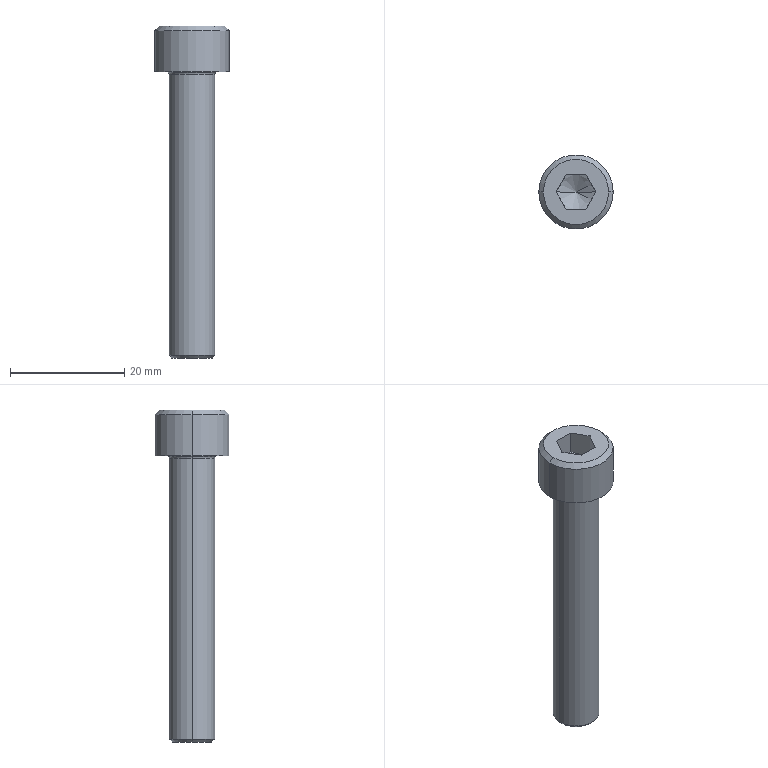Part | Creo | 1 solid | 23 faces | box 13 x 13 x 58 mm | volume 3411 mm3 | plane 9 | cone 6 | cylinder 4 | torus 4 | commonest cylinder face diameters 8 x2 13 x2
STEP:
#1=CARTESIAN_POINT('',(-230.536,192.995,-16.));
#2=VERTEX_POINT('',#1);
#3=CARTESIAN_POINT('',(-232.268,195.995,-16.));
#4=VERTEX_POINT('',#3);
#5=CARTESIAN_POINT('',(-230.536,192.995,-16.));
#6=CARTESIAN_POINT('',(-230.587,193.083,-16.029));
#7=CARTESIAN_POINT('',(-230.686,193.256,-16.083));
#8=CARTESIAN_POINT('',(-230.831,193.506,-16.149));
#9=CARTESIAN_POINT('',(-230.973,193.752,-16.201));
#10=CARTESIAN_POINT('',(-231.114,193.997,-16.239));
#11=CARTESIAN_POINT('',(-231.258,194.246,-16.263));
#12=CARTESIAN_POINT('',(-231.402,194.495,-16.271));
#13=CARTESIAN_POINT('',(-231.546,194.745,-16.263));
#14=CARTESIAN_POINT('',(-231.689,194.993,-16.239));
#15=CARTESIAN_POINT('',(-231.831,195.238,-16.201));
#16=CARTESIAN_POINT('',(-231.973,195.484,-16.149));
#17=CARTESIAN_POINT('',(-232.117,195.735,-16.083));
#18=CARTESIAN_POINT('',(-232.217,195.908,-16.029));
#19=CARTESIAN_POINT('',(-232.268,195.995,-16.));
#20=B_SPLINE_CURVE_WITH_KNOTS('',3,(#5,#6,#7,#8,#9,#10,#11,#12,#13,#14,#15,#16,#17,#18,#19),.UNSPECIFIED.,.F.,.F.,(4,1,1,1,1,1,1,1,1,1,1,1,4),(0.,0.08333,0.1667,0.25,0.3333,0.4167,0.5,0.5833,0.6667,0.75,0.8333,0.9167,1.),.UNSPECIFIED.);
#21=EDGE_CURVE('',#2,#4,#20,.T.);
#22=ORIENTED_EDGE('',*,*,#21,.F.);
#23=CARTESIAN_POINT('',(-234.,192.995,-18.));
#24=VERTEX_POINT('',#23);
#25=CARTESIAN_POINT('',(-234.,192.995,-18.));
#26=DIRECTION('',(0.866,0.,0.5));
#27=VECTOR('',#26,4.);
#28=LINE('',#25,#27);
#29=EDGE_CURVE('',#24,#2,#28,.T.);
#30=ORIENTED_EDGE('',*,*,#29,.F.);
#31=CARTESIAN_POINT('',(-237.464,192.995,-16.));
#32=VERTEX_POINT('',#31);
#33=CARTESIAN_POINT('',(-234.,192.995,-18.));
#34=DIRECTION('',(-0.866,0.,0.5));
#35=VECTOR('',#34,4.);
#36=LINE('',#33,#35);
#37=EDGE_CURVE('',#24,#32,#36,.T.);
#38=ORIENTED_EDGE('',*,*,#37,.T.);
#39=CARTESIAN_POINT('',(-235.732,195.995,-16.));
#40=VERTEX_POINT('',#39);
#41=CARTESIAN_POINT('',(-235.732,195.995,-16.));
#42=CARTESIAN_POINT('',(-235.783,195.908,-16.029));
#43=CARTESIAN_POINT('',(-235.883,195.735,-16.083));
#44=CARTESIAN_POINT('',(-236.027,195.484,-16.149));
#45=CARTESIAN_POINT('',(-236.169,195.238,-16.201));
#46=CARTESIAN_POINT('',(-236.311,194.993,-16.239));
#47=CARTESIAN_POINT('',(-236.454,194.745,-16.263));
#48=CARTESIAN_POINT('',(-236.598,194.495,-16.271));
#49=CARTESIAN_POINT('',(-236.742,194.246,-16.263));
#50=CARTESIAN_POINT('',(-236.886,193.997,-16.239));
#51=CARTESIAN_POINT('',(-237.027,193.752,-16.201));
#52=CARTESIAN_POINT('',(-237.169,193.506,-16.149));
#53=CARTESIAN_POINT('',(-237.314,193.256,-16.083));
#54=CARTESIAN_POINT('',(-237.413,193.083,-16.029));
#55=CARTESIAN_POINT('',(-237.464,192.995,-16.));
#56=B_SPLINE_CURVE_WITH_KNOTS('',3,(#41,#42,#43,#44,#45,#46,#47,#48,#49,#50,#51,#52,#53,#54,#55),.UNSPECIFIED.,.F.,.F.,(4,1,1,1,1,1,1,1,1,1,1,1,4),(0.,0.08333,0.1667,0.25,0.3333,0.4167,0.5,0.5833,0.6667,0.75,0.8333,0.9167,1.),.UNSPECIFIED.);
#57=EDGE_CURVE('',#40,#32,#56,.T.);
#58=ORIENTED_EDGE('',*,*,#57,.F.);
#59=CARTESIAN_POINT('',(-232.268,195.995,-16.));
#60=CARTESIAN_POINT('',(-232.369,195.995,-16.029));
#61=CARTESIAN_POINT('',(-232.569,195.995,-16.083));
#62=CARTESIAN_POINT('',(-232.857,195.995,-16.149));
#63=CARTESIAN_POINT('',(-233.141,195.995,-16.201));
#64=CARTESIAN_POINT('',(-233.424,195.995,-16.239));
#65=CARTESIAN_POINT('',(-233.711,195.995,-16.263));
#66=CARTESIAN_POINT('',(-234.,195.995,-16.271));
#67=CARTESIAN_POINT('',(-234.289,195.995,-16.263));
#68=CARTESIAN_POINT('',(-234.576,195.995,-16.239));
#69=CARTESIAN_POINT('',(-234.859,195.995,-16.201));
#70=CARTESIAN_POINT('',(-235.143,195.995,-16.149));
#71=CARTESIAN_POINT('',(-235.431,195.995,-16.083));
#72=CARTESIAN_POINT('',(-235.631,195.995,-16.029));
#73=CARTESIAN_POINT('',(-235.732,195.995,-16.));
#74=B_SPLINE_CURVE_WITH_KNOTS('',3,(#59,#60,#61,#62,#63,#64,#65,#66,#67,#68,#69,#70,#71,#72,#73),.UNSPECIFIED.,.F.,.F.,(4,1,1,1,1,1,1,1,1,1,1,1,4),(0.,0.08333,0.1667,0.25,0.3333,0.4167,0.5,0.5833,0.6667,0.75,0.8333,0.9167,1.),.UNSPECIFIED.);
#75=EDGE_CURVE('',#4,#40,#74,.T.);
#76=ORIENTED_EDGE('',*,*,#75,.F.);
#77=EDGE_LOOP('',(#22,#30,#38,#58,#76));
#78=FACE_OUTER_BOUND('',#77,.F.);
#79=CARTESIAN_POINT('',(-234.,192.995,-16.98));
#80=DIRECTION('',(0.,0.,1.));
#81=DIRECTION('',(1.,0.,0.));
#82=AXIS2_PLACEMENT_3D('',#79,#80,#81);
#83=CONICAL_SURFACE('',#82,1.767,60.);
#84=ADVANCED_FACE('',(#78),#83,.F.);
#85=CARTESIAN_POINT('',(-232.268,195.995,-12.));
#86=VERTEX_POINT('',#85);
#87=CARTESIAN_POINT('',(-230.536,192.995,-12.));
#88=VERTEX_POINT('',#87);
#89=CARTESIAN_POINT('',(-232.268,195.995,-12.));
#90=DIRECTION('',(0.5,-0.866,0.));
#91=VECTOR('',#90,3.464);
#92=LINE('',#89,#91);
#93=EDGE_CURVE('',#86,#88,#92,.T.);
#94=ORIENTED_EDGE('',*,*,#93,.T.);
#95=CARTESIAN_POINT('',(-230.536,192.995,-12.));
#96=DIRECTION('',(0.,0.,-1.));
#97=VECTOR('',#96,4.);
#98=LINE('',#95,#97);
#99=EDGE_CURVE('',#88,#2,#98,.T.);
#100=ORIENTED_EDGE('',*,*,#99,.T.);
#101=ORIENTED_EDGE('',*,*,#21,.T.);
#102=CARTESIAN_POINT('',(-232.268,195.995,-12.));
#103=DIRECTION('',(0.,0.,-1.));
#104=VECTOR('',#103,4.);
#105=LINE('',#102,#104);
#106=EDGE_CURVE('',#86,#4,#105,.T.);
#107=ORIENTED_EDGE('',*,*,#106,.F.);
#108=EDGE_LOOP('',(#94,#100,#101,#107));
#109=FACE_OUTER_BOUND('',#108,.F.);
#110=CARTESIAN_POINT('',(-232.268,195.995,-16.));
#111=DIRECTION('',(-0.866,-0.5,0.));
#112=DIRECTION('',(0.5,-0.866,0.));
#113=AXIS2_PLACEMENT_3D('',#110,#111,#112);
#114=PLANE('',#113);
#115=ADVANCED_FACE('',(#109),#114,.T.);
#116=CARTESIAN_POINT('',(-228.3,192.995,-12.));
#117=VERTEX_POINT('',#116);
#118=CARTESIAN_POINT('',(-239.7,192.995,-12.));
#119=VERTEX_POINT('',#118);
#120=CARTESIAN_POINT('',(-234.,192.995,-12.));
#121=DIRECTION('',(0.,0.,1.));
#122=DIRECTION('',(1.,0.,0.));
#123=AXIS2_PLACEMENT_3D('',#120,#121,#122);
#124=CIRCLE('',#123,5.7);
#125=EDGE_CURVE('',#117,#119,#124,.T.);
#126=ORIENTED_EDGE('',*,*,#125,.F.);
#127=CARTESIAN_POINT('',(-234.,192.995,-12.));
#128=DIRECTION('',(0.,0.,1.));
#129=DIRECTION('',(-1.,0.,0.));
#130=AXIS2_PLACEMENT_3D('',#127,#128,#129);
#131=CIRCLE('',#130,5.7);
#132=EDGE_CURVE('',#119,#117,#131,.T.);
#133=ORIENTED_EDGE('',*,*,#132,.F.);
#134=EDGE_LOOP('',(#126,#133));
#135=FACE_OUTER_BOUND('',#134,.F.);
#136=CARTESIAN_POINT('',(-232.268,189.995,-12.));
#137=VERTEX_POINT('',#136);
#138=CARTESIAN_POINT('',(-230.536,192.995,-12.));
#139=DIRECTION('',(-0.5,-0.866,0.));
#140=VECTOR('',#139,3.464);
#141=LINE('',#138,#140);
#142=EDGE_CURVE('',#88,#137,#141,.T.);
#143=ORIENTED_EDGE('',*,*,#142,.F.);
#144=ORIENTED_EDGE('',*,*,#93,.F.);
#145=CARTESIAN_POINT('',(-235.732,195.995,-12.));
#146=VERTEX_POINT('',#145);
#147=CARTESIAN_POINT('',(-232.268,195.995,-12.));
#148=DIRECTION('',(-1.,0.,0.));
#149=VECTOR('',#148,3.464);
#150=LINE('',#147,#149);
#151=EDGE_CURVE('',#86,#146,#150,.T.);
#152=ORIENTED_EDGE('',*,*,#151,.T.);
#153=CARTESIAN_POINT('',(-237.464,192.995,-12.));
#154=VERTEX_POINT('',#153);
#155=CARTESIAN_POINT('',(-237.464,192.995,-12.));
#156=DIRECTION('',(0.5,0.866,0.));
#157=VECTOR('',#156,3.464);
#158=LINE('',#155,#157);
#159=EDGE_CURVE('',#154,#146,#158,.T.);
#160=ORIENTED_EDGE('',*,*,#159,.F.);
#161=CARTESIAN_POINT('',(-235.732,189.995,-12.));
#162=VERTEX_POINT('',#161);
#163=CARTESIAN_POINT('',(-235.732,189.995,-12.));
#164=DIRECTION('',(-0.5,0.866,0.));
#165=VECTOR('',#164,3.464);
#166=LINE('',#163,#165);
#167=EDGE_CURVE('',#162,#154,#166,.T.);
#168=ORIENTED_EDGE('',*,*,#167,.F.);
#169=CARTESIAN_POINT('',(-235.732,189.995,-12.));
#170=DIRECTION('',(1.,0.,0.));
#171=VECTOR('',#170,3.464);
#172=LINE('',#169,#171);
#173=EDGE_CURVE('',#162,#137,#172,.T.);
#174=ORIENTED_EDGE('',*,*,#173,.T.);
#175=EDGE_LOOP('',(#143,#144,#152,#160,#168,#174));
#176=FACE_BOUND('',#175,.F.);
#177=CARTESIAN_POINT('',(-234.,192.995,-12.));
#178=DIRECTION('',(0.,0.,1.));
#179=DIRECTION('',(1.,0.,0.));
#180=AXIS2_PLACEMENT_3D('',#177,#178,#179);
#181=PLANE('',#180);
#182=ADVANCED_FACE('',(#135,#176),#181,.T.);
#183=CARTESIAN_POINT('',(-227.5,192.995,-12.8));
#184=VERTEX_POINT('',#183);
#185=CARTESIAN_POINT('',(-240.5,192.995,-12.8));
#186=VERTEX_POINT('',#185);
#187=CARTESIAN_POINT('',(-234.,192.995,-12.8));
#188=DIRECTION('',(0.,0.,1.));
#189=DIRECTION('',(1.,0.,0.));
#190=AXIS2_PLACEMENT_3D('',#187,#188,#189);
#191=CIRCLE('',#190,6.5);
#192=EDGE_CURVE('',#184,#186,#191,.T.);
#193=ORIENTED_EDGE('',*,*,#192,.F.);
#194=CARTESIAN_POINT('',(-228.3,192.995,-12.));
#195=DIRECTION('',(0.7071,0.,-0.7071));
#196=VECTOR('',#195,1.131);
#197=LINE('',#194,#196);
#198=EDGE_CURVE('',#117,#184,#197,.T.);
#199=ORIENTED_EDGE('',*,*,#198,.F.);
#200=ORIENTED_EDGE('',*,*,#125,.T.);
#201=CARTESIAN_POINT('',(-239.7,192.995,-12.));
#202=DIRECTION('',(-0.7071,0.,-0.7071));
#203=VECTOR('',#202,1.131);
#204=LINE('',#201,#203);
#205=EDGE_CURVE('',#119,#186,#204,.T.);
#206=ORIENTED_EDGE('',*,*,#205,.T.);
#207=EDGE_LOOP('',(#193,#199,#200,#206));
#208=FACE_OUTER_BOUND('',#207,.F.);
#209=CARTESIAN_POINT('',(-234.,192.995,-12.4));
#210=DIRECTION('',(0.,0.,-1.));
#211=DIRECTION('',(-1.,0.,0.));
#212=AXIS2_PLACEMENT_3D('',#209,#210,#211);
#213=CONICAL_SURFACE('',#212,6.1,45.);
#214=ADVANCED_FACE('',(#208),#213,.T.);
#215=ORIENTED_EDGE('',*,*,#192,.T.);
#216=CARTESIAN_POINT('',(-240.5,192.995,-20.));
#217=VERTEX_POINT('',#216);
#218=CARTESIAN_POINT('',(-240.5,192.995,-20.));
#219=DIRECTION('',(0.,0.,1.));
#220=VECTOR('',#219,7.2);
#221=LINE('',#218,#220);
#222=EDGE_CURVE('',#217,#186,#221,.T.);
#223=ORIENTED_EDGE('',*,*,#222,.F.);
#224=CARTESIAN_POINT('',(-227.5,192.995,-20.));
#225=VERTEX_POINT('',#224);
#226=CARTESIAN_POINT('',(-234.,192.995,-20.));
#227=DIRECTION('',(0.,0.,-1.));
#228=DIRECTION('',(-1.,0.,0.));
#229=AXIS2_PLACEMENT_3D('',#226,#227,#228);
#230=CIRCLE('',#229,6.5);
#231=EDGE_CURVE('',#217,#225,#230,.T.);
#232=ORIENTED_EDGE('',*,*,#231,.T.);
#233=CARTESIAN_POINT('',(-227.5,192.995,-20.));
#234=DIRECTION('',(0.,0.,1.));
#235=VECTOR('',#234,7.2);
#236=LINE('',#233,#235);
#237=EDGE_CURVE('',#225,#184,#236,.T.);
#238=ORIENTED_EDGE('',*,*,#237,.T.);
#239=EDGE_LOOP('',(#215,#223,#232,#238));
#240=FACE_OUTER_BOUND('',#239,.F.);
#241=CARTESIAN_POINT('',(-234.,192.995,-20.));
#242=DIRECTION('',(0.,0.,1.));
#243=DIRECTION('',(1.,0.,0.));
#244=AXIS2_PLACEMENT_3D('',#241,#242,#243);
#245=CYLINDRICAL_SURFACE('',#244,6.5);
#246=ADVANCED_FACE('',(#240),#245,.T.);
#247=CARTESIAN_POINT('',(-234.,192.995,-12.8));
#248=DIRECTION('',(0.,0.,1.));
#249=DIRECTION('',(-1.,0.,0.));
#250=AXIS2_PLACEMENT_3D('',#247,#248,#249);
#251=CIRCLE('',#250,6.5);
#252=EDGE_CURVE('',#186,#184,#251,.T.);
#253=ORIENTED_EDGE('',*,*,#252,.T.);
#254=ORIENTED_EDGE('',*,*,#237,.F.);
#255=CARTESIAN_POINT('',(-234.,192.995,-20.));
#256=DIRECTION('',(0.,0.,-1.));
#257=DIRECTION('',(1.,0.,0.));
#258=AXIS2_PLACEMENT_3D('',#255,#256,#257);
#259=CIRCLE('',#258,6.5);
#260=EDGE_CURVE('',#225,#217,#259,.T.);
#261=ORIENTED_EDGE('',*,*,#260,.T.);
#262=ORIENTED_EDGE('',*,*,#222,.T.);
#263=EDGE_LOOP('',(#253,#254,#261,#262));
#264=FACE_OUTER_BOUND('',#263,.F.);
#265=CARTESIAN_POINT('',(-234.,192.995,-20.));
#266=DIRECTION('',(0.,0.,1.));
#267=DIRECTION('',(1.,0.,0.));
#268=AXIS2_PLACEMENT_3D('',#265,#266,#267);
#269=CYLINDRICAL_SURFACE('',#268,6.5);
#270=ADVANCED_FACE('',(#264),#269,.T.);
#271=ORIENTED_EDGE('',*,*,#252,.F.);
#272=ORIENTED_EDGE('',*,*,#205,.F.);
#273=ORIENTED_EDGE('',*,*,#132,.T.);
#274=ORIENTED_EDGE('',*,*,#198,.T.);
#275=EDGE_LOOP('',(#271,#272,#273,#274));
#276=FACE_OUTER_BOUND('',#275,.F.);
#277=CARTESIAN_POINT('',(-234.,192.995,-12.4));
#278=DIRECTION('',(0.,0.,-1.));
#279=DIRECTION('',(-1.,0.,0.));
#280=AXIS2_PLACEMENT_3D('',#277,#278,#279);
#281=CONICAL_SURFACE('',#280,6.1,45.);
#282=ADVANCED_FACE('',(#276),#281,.T.);
#283=ORIENTED_EDGE('',*,*,#260,.F.);
#284=ORIENTED_EDGE('',*,*,#231,.F.);
#285=EDGE_LOOP('',(#283,#284));
#286=FACE_OUTER_BOUND('',#285,.F.);
#287=CARTESIAN_POINT('',(-229.6,192.995,-20.));
#288=VERTEX_POINT('',#287);
#289=CARTESIAN_POINT('',(-238.4,192.995,-20.));
#290=VERTEX_POINT('',#289);
#291=CARTESIAN_POINT('',(-234.,192.995,-20.));
#292=DIRECTION('',(0.,0.,1.));
#293=DIRECTION('',(1.,0.,0.));
#294=AXIS2_PLACEMENT_3D('',#291,#292,#293);
#295=CIRCLE('',#294,4.4);
#296=EDGE_CURVE('',#288,#290,#295,.T.);
#297=ORIENTED_EDGE('',*,*,#296,.F.);
#298=CARTESIAN_POINT('',(-234.,192.995,-20.));
#299=DIRECTION('',(0.,0.,1.));
#300=DIRECTION('',(-1.,0.,0.));
#301=AXIS2_PLACEMENT_3D('',#298,#299,#300);
#302=CIRCLE('',#301,4.4);
#303=EDGE_CURVE('',#290,#288,#302,.T.);
#304=ORIENTED_EDGE('',*,*,#303,.F.);
#305=EDGE_LOOP('',(#297,#304));
#306=FACE_BOUND('',#305,.F.);
#307=CARTESIAN_POINT('',(-234.,192.995,-20.));
#308=DIRECTION('',(0.,0.,1.));
#309=DIRECTION('',(1.,0.,0.));
#310=AXIS2_PLACEMENT_3D('',#307,#308,#309);
#311=PLANE('',#310);
#312=ADVANCED_FACE('',(#286,#306),#311,.F.);
#313=ORIENTED_EDGE('',*,*,#296,.T.);
#314=CARTESIAN_POINT('',(-238.117,192.995,-20.117));
#315=VERTEX_POINT('',#314);
#316=CARTESIAN_POINT('',(-238.4,192.995,-20.4));
#317=DIRECTION('',(0.,1.,0.));
#318=DIRECTION('',(0.,0.,1.));
#319=AXIS2_PLACEMENT_3D('',#316,#317,#318);
#320=CIRCLE('',#319,0.4);
#321=EDGE_CURVE('',#290,#315,#320,.T.);
#322=ORIENTED_EDGE('',*,*,#321,.T.);
#323=CARTESIAN_POINT('',(-229.883,192.995,-20.117));
#324=VERTEX_POINT('',#323);
#325=CARTESIAN_POINT('',(-234.,192.995,-20.117));
#326=DIRECTION('',(0.,0.,1.));
#327=DIRECTION('',(1.,0.,0.));
#328=AXIS2_PLACEMENT_3D('',#325,#326,#327);
#329=CIRCLE('',#328,4.117);
#330=EDGE_CURVE('',#324,#315,#329,.T.);
#331=ORIENTED_EDGE('',*,*,#330,.F.);
#332=CARTESIAN_POINT('',(-229.6,192.995,-20.4));
#333=DIRECTION('',(0.,-1.,0.));
#334=DIRECTION('',(0.,0.,1.));
#335=AXIS2_PLACEMENT_3D('',#332,#333,#334);
#336=CIRCLE('',#335,0.4);
#337=EDGE_CURVE('',#288,#324,#336,.T.);
#338=ORIENTED_EDGE('',*,*,#337,.F.);
#339=EDGE_LOOP('',(#313,#322,#331,#338));
#340=FACE_OUTER_BOUND('',#339,.F.);
#341=CARTESIAN_POINT('',(-234.,192.995,-20.4));
#342=DIRECTION('',(0.,0.,1.));
#343=DIRECTION('',(1.,0.,0.));
#344=AXIS2_PLACEMENT_3D('',#341,#342,#343);
#345=TOROIDAL_SURFACE('',#344,4.4,0.4);
#346=ADVANCED_FACE('',(#340),#345,.F.);
#347=ORIENTED_EDGE('',*,*,#303,.T.);
#348=ORIENTED_EDGE('',*,*,#337,.T.);
#349=CARTESIAN_POINT('',(-234.,192.995,-20.117));
#350=DIRECTION('',(0.,0.,1.));
#351=DIRECTION('',(-1.,0.,0.));
#352=AXIS2_PLACEMENT_3D('',#349,#350,#351);
#353=CIRCLE('',#352,4.117);
#354=EDGE_CURVE('',#315,#324,#353,.T.);
#355=ORIENTED_EDGE('',*,*,#354,.F.);
#356=ORIENTED_EDGE('',*,*,#321,.F.);
#357=EDGE_LOOP('',(#347,#348,#355,#356));
#358=FACE_OUTER_BOUND('',#357,.F.);
#359=CARTESIAN_POINT('',(-234.,192.995,-20.4));
#360=DIRECTION('',(0.,0.,1.));
#361=DIRECTION('',(1.,0.,0.));
#362=AXIS2_PLACEMENT_3D('',#359,#360,#361);
#363=TOROIDAL_SURFACE('',#362,4.4,0.4);
#364=ADVANCED_FACE('',(#358),#363,.F.);
#365=CARTESIAN_POINT('',(-238.,192.995,-20.4));
#366=VERTEX_POINT('',#365);
#367=CARTESIAN_POINT('',(-230.,192.995,-20.4));
#368=VERTEX_POINT('',#367);
#369=CARTESIAN_POINT('',(-234.,192.995,-20.4));
#370=DIRECTION('',(0.,0.,1.));
#371=DIRECTION('',(-1.,0.,0.));
#372=AXIS2_PLACEMENT_3D('',#369,#370,#371);
#373=CIRCLE('',#372,4.);
#374=EDGE_CURVE('',#366,#368,#373,.T.);
#375=ORIENTED_EDGE('',*,*,#374,.F.);
#376=CARTESIAN_POINT('',(-238.4,192.995,-20.4));
#377=DIRECTION('',(0.,1.,0.));
#378=DIRECTION('',(0.7071,0.,0.7071));
#379=AXIS2_PLACEMENT_3D('',#376,#377,#378);
#380=CIRCLE('',#379,0.4);
#381=EDGE_CURVE('',#315,#366,#380,.T.);
#382=ORIENTED_EDGE('',*,*,#381,.F.);
#383=ORIENTED_EDGE('',*,*,#354,.T.);
#384=CARTESIAN_POINT('',(-229.6,192.995,-20.4));
#385=DIRECTION('',(0.,-1.,0.));
#386=DIRECTION('',(-0.7071,0.,0.7071));
#387=AXIS2_PLACEMENT_3D('',#384,#385,#386);
#388=CIRCLE('',#387,0.4);
#389=EDGE_CURVE('',#324,#368,#388,.T.);
#390=ORIENTED_EDGE('',*,*,#389,.T.);
#391=EDGE_LOOP('',(#375,#382,#383,#390));
#392=FACE_OUTER_BOUND('',#391,.F.);
#393=CARTESIAN_POINT('',(-234.,192.995,-20.4));
#394=DIRECTION('',(0.,0.,1.));
#395=DIRECTION('',(1.,0.,0.));
#396=AXIS2_PLACEMENT_3D('',#393,#394,#395);
#397=TOROIDAL_SURFACE('',#396,4.4,0.4);
#398=ADVANCED_FACE('',(#392),#397,.F.);
#399=CARTESIAN_POINT('',(-230.,192.995,-69.5));
#400=VERTEX_POINT('',#399);
#401=CARTESIAN_POINT('',(-238.,192.995,-69.5));
#402=VERTEX_POINT('',#401);
#403=CARTESIAN_POINT('',(-234.,192.995,-69.5));
#404=DIRECTION('',(0.,0.,-1.));
#405=DIRECTION('',(1.,0.,0.));
#406=AXIS2_PLACEMENT_3D('',#403,#404,#405);
#407=CIRCLE('',#406,4.);
#408=EDGE_CURVE('',#400,#402,#407,.T.);
#409=ORIENTED_EDGE('',*,*,#408,.T.);
#410=CARTESIAN_POINT('',(-238.,192.995,-69.5));
#411=DIRECTION('',(0.,0.,1.));
#412=VECTOR('',#411,49.1);
#413=LINE('',#410,#412);
#414=EDGE_CURVE('',#402,#366,#413,.T.);
#415=ORIENTED_EDGE('',*,*,#414,.T.);
#416=ORIENTED_EDGE('',*,*,#374,.T.);
#417=CARTESIAN_POINT('',(-230.,192.995,-69.5));
#418=DIRECTION('',(0.,0.,1.));
#419=VECTOR('',#418,49.1);
#420=LINE('',#417,#419);
#421=EDGE_CURVE('',#400,#368,#420,.T.);
#422=ORIENTED_EDGE('',*,*,#421,.F.);
#423=EDGE_LOOP('',(#409,#415,#416,#422));
#424=FACE_OUTER_BOUND('',#423,.F.);
#425=CARTESIAN_POINT('',(-234.,192.995,-70.));
#426=DIRECTION('',(0.,0.,1.));
#427=DIRECTION('',(1.,0.,0.));
#428=AXIS2_PLACEMENT_3D('',#425,#426,#427);
#429=CYLINDRICAL_SURFACE('',#428,4.);
#430=ADVANCED_FACE('',(#424),#429,.T.);
#431=CARTESIAN_POINT('',(-230.5,192.995,-70.));
#432=VERTEX_POINT('',#431);
#433=CARTESIAN_POINT('',(-237.5,192.995,-70.));
#434=VERTEX_POINT('',#433);
#435=CARTESIAN_POINT('',(-234.,192.995,-70.));
#436=DIRECTION('',(0.,0.,-1.));
#437=DIRECTION('',(1.,0.,0.));
#438=AXIS2_PLACEMENT_3D('',#435,#436,#437);
#439=CIRCLE('',#438,3.5);
#440=EDGE_CURVE('',#432,#434,#439,.T.);
#441=ORIENTED_EDGE('',*,*,#440,.T.);
#442=CARTESIAN_POINT('',(-237.5,192.995,-70.));
#443=DIRECTION('',(-0.7071,0.,0.7071));
#444=VECTOR('',#443,0.7071);
#445=LINE('',#442,#444);
#446=EDGE_CURVE('',#434,#402,#445,.T.);
#447=ORIENTED_EDGE('',*,*,#446,.T.);
#448=ORIENTED_EDGE('',*,*,#408,.F.);
#449=CARTESIAN_POINT('',(-230.5,192.995,-70.));
#450=DIRECTION('',(0.7071,0.,0.7071));
#451=VECTOR('',#450,0.7071);
#452=LINE('',#449,#451);
#453=EDGE_CURVE('',#432,#400,#452,.T.);
#454=ORIENTED_EDGE('',*,*,#453,.F.);
#455=EDGE_LOOP('',(#441,#447,#448,#454));
#456=FACE_OUTER_BOUND('',#455,.F.);
#457=CARTESIAN_POINT('',(-234.,192.995,-69.75));
#458=DIRECTION('',(0.,0.,1.));
#459=DIRECTION('',(1.,0.,0.));
#460=AXIS2_PLACEMENT_3D('',#457,#458,#459);
#461=CONICAL_SURFACE('',#460,3.75,45.);
#462=ADVANCED_FACE('',(#456),#461,.T.);
#463=ORIENTED_EDGE('',*,*,#440,.F.);
#464=CARTESIAN_POINT('',(-234.,192.995,-70.));
#465=DIRECTION('',(0.,0.,-1.));
#466=DIRECTION('',(-1.,0.,0.));
#467=AXIS2_PLACEMENT_3D('',#464,#465,#466);
#468=CIRCLE('',#467,3.5);
#469=EDGE_CURVE('',#434,#432,#468,.T.);
#470=ORIENTED_EDGE('',*,*,#469,.F.);
#471=EDGE_LOOP('',(#463,#470));
#472=FACE_OUTER_BOUND('',#471,.F.);
#473=CARTESIAN_POINT('',(-234.,192.995,-70.));
#474=DIRECTION('',(0.,0.,1.));
#475=DIRECTION('',(1.,0.,0.));
#476=AXIS2_PLACEMENT_3D('',#473,#474,#475);
#477=PLANE('',#476);
#478=ADVANCED_FACE('',(#472),#477,.F.);
#479=ORIENTED_EDGE('',*,*,#469,.T.);
#480=ORIENTED_EDGE('',*,*,#453,.T.);
#481=CARTESIAN_POINT('',(-234.,192.995,-69.5));
#482=DIRECTION('',(0.,0.,-1.));
#483=DIRECTION('',(-1.,0.,0.));
#484=AXIS2_PLACEMENT_3D('',#481,#482,#483);
#485=CIRCLE('',#484,4.);
#486=EDGE_CURVE('',#402,#400,#485,.T.);
#487=ORIENTED_EDGE('',*,*,#486,.F.);
#488=ORIENTED_EDGE('',*,*,#446,.F.);
#489=EDGE_LOOP('',(#479,#480,#487,#488));
#490=FACE_OUTER_BOUND('',#489,.F.);
#491=CARTESIAN_POINT('',(-234.,192.995,-69.75));
#492=DIRECTION('',(0.,0.,1.));
#493=DIRECTION('',(1.,0.,0.));
#494=AXIS2_PLACEMENT_3D('',#491,#492,#493);
#495=CONICAL_SURFACE('',#494,3.75,45.);
#496=ADVANCED_FACE('',(#490),#495,.T.);
#497=ORIENTED_EDGE('',*,*,#486,.T.);
#498=ORIENTED_EDGE('',*,*,#421,.T.);
#499=CARTESIAN_POINT('',(-234.,192.995,-20.4));
#500=DIRECTION('',(0.,0.,1.));
#501=DIRECTION('',(1.,0.,0.));
#502=AXIS2_PLACEMENT_3D('',#499,#500,#501);
#503=CIRCLE('',#502,4.);
#504=EDGE_CURVE('',#368,#366,#503,.T.);
#505=ORIENTED_EDGE('',*,*,#504,.T.);
#506=ORIENTED_EDGE('',*,*,#414,.F.);
#507=EDGE_LOOP('',(#497,#498,#505,#506));
#508=FACE_OUTER_BOUND('',#507,.F.);
#509=CARTESIAN_POINT('',(-234.,192.995,-70.));
#510=DIRECTION('',(0.,0.,1.));
#511=DIRECTION('',(1.,0.,0.));
#512=AXIS2_PLACEMENT_3D('',#509,#510,#511);
#513=CYLINDRICAL_SURFACE('',#512,4.);
#514=ADVANCED_FACE('',(#508),#513,.T.);
#515=ORIENTED_EDGE('',*,*,#504,.F.);
#516=ORIENTED_EDGE('',*,*,#389,.F.);
#517=ORIENTED_EDGE('',*,*,#330,.T.);
#518=ORIENTED_EDGE('',*,*,#381,.T.);
#519=EDGE_LOOP('',(#515,#516,#517,#518));
#520=FACE_OUTER_BOUND('',#519,.F.);
#521=CARTESIAN_POINT('',(-234.,192.995,-20.4));
#522=DIRECTION('',(0.,0.,1.));
#523=DIRECTION('',(1.,0.,0.));
#524=AXIS2_PLACEMENT_3D('',#521,#522,#523);
#525=TOROIDAL_SURFACE('',#524,4.4,0.4);
#526=ADVANCED_FACE('',(#520),#525,.F.);
#527=ORIENTED_EDGE('',*,*,#142,.T.);
#528=CARTESIAN_POINT('',(-232.268,189.995,-16.));
#529=VERTEX_POINT('',#528);
#530=CARTESIAN_POINT('',(-232.268,189.995,-12.));
#531=DIRECTION('',(0.,0.,-1.));
#532=VECTOR('',#531,4.);
#533=LINE('',#530,#532);
#534=EDGE_CURVE('',#137,#529,#533,.T.);
#535=ORIENTED_EDGE('',*,*,#534,.T.);
#536=CARTESIAN_POINT('',(-232.268,189.995,-16.));
#537=CARTESIAN_POINT('',(-232.217,190.083,-16.029));
#538=CARTESIAN_POINT('',(-232.117,190.256,-16.083));
#539=CARTESIAN_POINT('',(-231.973,190.506,-16.149));
#540=CARTESIAN_POINT('',(-231.831,190.752,-16.201));
#541=CARTESIAN_POINT('',(-231.689,190.997,-16.239));
#542=CARTESIAN_POINT('',(-231.546,191.246,-16.263));
#543=CARTESIAN_POINT('',(-231.402,191.495,-16.271));
#544=CARTESIAN_POINT('',(-231.258,191.745,-16.263));
#545=CARTESIAN_POINT('',(-231.114,191.993,-16.239));
#546=CARTESIAN_POINT('',(-230.973,192.238,-16.201));
#547=CARTESIAN_POINT('',(-230.831,192.484,-16.149));
#548=CARTESIAN_POINT('',(-230.686,192.735,-16.083));
#549=CARTESIAN_POINT('',(-230.587,192.908,-16.029));
#550=CARTESIAN_POINT('',(-230.536,192.995,-16.));
#551=B_SPLINE_CURVE_WITH_KNOTS('',3,(#536,#537,#538,#539,#540,#541,#542,#543,#544,#545,#546,#547,#548,#549,#550),.UNSPECIFIED.,.F.,.F.,(4,1,1,1,1,1,1,1,1,1,1,1,4),(0.,0.08333,0.1667,0.25,0.3333,0.4167,0.5,0.5833,0.6667,0.75,0.8333,0.9167,1.),.UNSPECIFIED.);
#552=EDGE_CURVE('',#529,#2,#551,.T.);
#553=ORIENTED_EDGE('',*,*,#552,.T.);
#554=ORIENTED_EDGE('',*,*,#99,.F.);
#555=EDGE_LOOP('',(#527,#535,#553,#554));
#556=FACE_OUTER_BOUND('',#555,.F.);
#557=CARTESIAN_POINT('',(-230.536,192.995,-16.));
#558=DIRECTION('',(-0.866,0.5,0.));
#559=DIRECTION('',(-0.5,-0.866,0.));
#560=AXIS2_PLACEMENT_3D('',#557,#558,#559);
#561=PLANE('',#560);
#562=ADVANCED_FACE('',(#556),#561,.T.);
#563=ORIENTED_EDGE('',*,*,#173,.F.);
#564=CARTESIAN_POINT('',(-235.732,189.995,-16.));
#565=VERTEX_POINT('',#564);
#566=CARTESIAN_POINT('',(-235.732,189.995,-12.));
#567=DIRECTION('',(0.,0.,-1.));
#568=VECTOR('',#567,4.);
#569=LINE('',#566,#568);
#570=EDGE_CURVE('',#162,#565,#569,.T.);
#571=ORIENTED_EDGE('',*,*,#570,.T.);
#572=CARTESIAN_POINT('',(-235.732,189.995,-16.));
#573=CARTESIAN_POINT('',(-235.631,189.995,-16.029));
#574=CARTESIAN_POINT('',(-235.431,189.995,-16.083));
#575=CARTESIAN_POINT('',(-235.143,189.995,-16.149));
#576=CARTESIAN_POINT('',(-234.859,189.995,-16.201));
#577=CARTESIAN_POINT('',(-234.576,189.995,-16.239));
#578=CARTESIAN_POINT('',(-234.289,189.995,-16.263));
#579=CARTESIAN_POINT('',(-234.,189.995,-16.271));
#580=CARTESIAN_POINT('',(-233.711,189.995,-16.263));
#581=CARTESIAN_POINT('',(-233.424,189.995,-16.239));
#582=CARTESIAN_POINT('',(-233.141,189.995,-16.201));
#583=CARTESIAN_POINT('',(-232.857,189.995,-16.149));
#584=CARTESIAN_POINT('',(-232.569,189.995,-16.083));
#585=CARTESIAN_POINT('',(-232.369,189.995,-16.029));
#586=CARTESIAN_POINT('',(-232.268,189.995,-16.));
#587=B_SPLINE_CURVE_WITH_KNOTS('',3,(#572,#573,#574,#575,#576,#577,#578,#579,#580,#581,#582,#583,#584,#585,#586),.UNSPECIFIED.,.F.,.F.,(4,1,1,1,1,1,1,1,1,1,1,1,4),(0.,0.08333,0.1667,0.25,0.3333,0.4167,0.5,0.5833,0.6667,0.75,0.8333,0.9167,1.),.UNSPECIFIED.);
#588=EDGE_CURVE('',#565,#529,#587,.T.);
#589=ORIENTED_EDGE('',*,*,#588,.T.);
#590=ORIENTED_EDGE('',*,*,#534,.F.);
#591=EDGE_LOOP('',(#563,#571,#589,#590));
#592=FACE_OUTER_BOUND('',#591,.F.);
#593=CARTESIAN_POINT('',(-232.268,189.995,-16.));
#594=DIRECTION('',(0.,1.,0.));
#595=DIRECTION('',(0.,0.,1.));
#596=AXIS2_PLACEMENT_3D('',#593,#594,#595);
#597=PLANE('',#596);
#598=ADVANCED_FACE('',(#592),#597,.T.);
#599=ORIENTED_EDGE('',*,*,#167,.T.);
#600=CARTESIAN_POINT('',(-237.464,192.995,-12.));
#601=DIRECTION('',(0.,0.,-1.));
#602=VECTOR('',#601,4.);
#603=LINE('',#600,#602);
#604=EDGE_CURVE('',#154,#32,#603,.T.);
#605=ORIENTED_EDGE('',*,*,#604,.T.);
#606=CARTESIAN_POINT('',(-237.464,192.995,-16.));
#607=CARTESIAN_POINT('',(-237.413,192.908,-16.029));
#608=CARTESIAN_POINT('',(-237.314,192.735,-16.083));
#609=CARTESIAN_POINT('',(-237.169,192.484,-16.149));
#610=CARTESIAN_POINT('',(-237.027,192.238,-16.201));
#611=CARTESIAN_POINT('',(-236.886,191.993,-16.239));
#612=CARTESIAN_POINT('',(-236.742,191.745,-16.263));
#613=CARTESIAN_POINT('',(-236.598,191.495,-16.271));
#614=CARTESIAN_POINT('',(-236.454,191.246,-16.263));
#615=CARTESIAN_POINT('',(-236.311,190.997,-16.239));
#616=CARTESIAN_POINT('',(-236.169,190.752,-16.201));
#617=CARTESIAN_POINT('',(-236.027,190.506,-16.149));
#618=CARTESIAN_POINT('',(-235.883,190.256,-16.083));
#619=CARTESIAN_POINT('',(-235.783,190.083,-16.029));
#620=CARTESIAN_POINT('',(-235.732,189.995,-16.));
#621=B_SPLINE_CURVE_WITH_KNOTS('',3,(#606,#607,#608,#609,#610,#611,#612,#613,#614,#615,#616,#617,#618,#619,#620),.UNSPECIFIED.,.F.,.F.,(4,1,1,1,1,1,1,1,1,1,1,1,4),(0.,0.08333,0.1667,0.25,0.3333,0.4167,0.5,0.5833,0.6667,0.75,0.8333,0.9167,1.),.UNSPECIFIED.);
#622=EDGE_CURVE('',#32,#565,#621,.T.);
#623=ORIENTED_EDGE('',*,*,#622,.T.);
#624=ORIENTED_EDGE('',*,*,#570,.F.);
#625=EDGE_LOOP('',(#599,#605,#623,#624));
#626=FACE_OUTER_BOUND('',#625,.F.);
#627=CARTESIAN_POINT('',(-235.732,189.995,-16.));
#628=DIRECTION('',(0.866,0.5,0.));
#629=DIRECTION('',(-0.5,0.866,0.));
#630=AXIS2_PLACEMENT_3D('',#627,#628,#629);
#631=PLANE('',#630);
#632=ADVANCED_FACE('',(#626),#631,.T.);
#633=ORIENTED_EDGE('',*,*,#159,.T.);
#634=CARTESIAN_POINT('',(-235.732,195.995,-12.));
#635=DIRECTION('',(0.,0.,-1.));
#636=VECTOR('',#635,4.);
#637=LINE('',#634,#636);
#638=EDGE_CURVE('',#146,#40,#637,.T.);
#639=ORIENTED_EDGE('',*,*,#638,.T.);
#640=ORIENTED_EDGE('',*,*,#57,.T.);
#641=ORIENTED_EDGE('',*,*,#604,.F.);
#642=EDGE_LOOP('',(#633,#639,#640,#641));
#643=FACE_OUTER_BOUND('',#642,.F.);
#644=CARTESIAN_POINT('',(-237.464,192.995,-16.));
#645=DIRECTION('',(0.866,-0.5,0.));
#646=DIRECTION('',(0.5,0.866,0.));
#647=AXIS2_PLACEMENT_3D('',#644,#645,#646);
#648=PLANE('',#647);
#649=ADVANCED_FACE('',(#643),#648,.T.);
#650=ORIENTED_EDGE('',*,*,#151,.F.);
#651=ORIENTED_EDGE('',*,*,#106,.T.);
#652=ORIENTED_EDGE('',*,*,#75,.T.);
#653=ORIENTED_EDGE('',*,*,#638,.F.);
#654=EDGE_LOOP('',(#650,#651,#652,#653));
#655=FACE_OUTER_BOUND('',#654,.F.);
#656=CARTESIAN_POINT('',(-235.732,195.995,-16.));
#657=DIRECTION('',(0.,-1.,0.));
#658=DIRECTION('',(0.,0.,-1.));
#659=AXIS2_PLACEMENT_3D('',#656,#657,#658);
#660=PLANE('',#659);
#661=ADVANCED_FACE('',(#655),#660,.T.);
#662=ORIENTED_EDGE('',*,*,#622,.F.);
#663=ORIENTED_EDGE('',*,*,#37,.F.);
#664=ORIENTED_EDGE('',*,*,#29,.T.);
#665=ORIENTED_EDGE('',*,*,#552,.F.);
#666=ORIENTED_EDGE('',*,*,#588,.F.);
#667=EDGE_LOOP('',(#662,#663,#664,#665,#666));
#668=FACE_OUTER_BOUND('',#667,.F.);
#669=CARTESIAN_POINT('',(-234.,192.995,-16.98));
#670=DIRECTION('',(0.,0.,1.));
#671=DIRECTION('',(1.,0.,0.));
#672=AXIS2_PLACEMENT_3D('',#669,#670,#671);
#673=CONICAL_SURFACE('',#672,1.767,60.);
#674=ADVANCED_FACE('',(#668),#673,.F.);
#675=CLOSED_SHELL('',(#84,#115,#182,#214,#246,#270,#282,#312,#346,#364,#398,#430,#462,#478,#496,#514,#526,#562,#598,#632,#649,#661,#674));
#676=MANIFOLD_SOLID_BREP('',#675);
#677=(LENGTH_UNIT()NAMED_UNIT(*)SI_UNIT(.MILLI.,.METRE.));
#678=UNCERTAINTY_MEASURE_WITH_UNIT(LENGTH_MEASURE(0.006085),#677,'','');
#679=(NAMED_UNIT(*)PLANE_ANGLE_UNIT()SI_UNIT($,.RADIAN.));
#680=PLANE_ANGLE_MEASURE_WITH_UNIT(PLANE_ANGLE_MEASURE(0.01745),#679);
#681=(CONVERSION_BASED_UNIT('DEGREE',#680)NAMED_UNIT(*)PLANE_ANGLE_UNIT());
#682=(NAMED_UNIT(*)SI_UNIT($,.STERADIAN.)SOLID_ANGLE_UNIT());
#683=(GEOMETRIC_REPRESENTATION_CONTEXT(3)GLOBAL_UNCERTAINTY_ASSIGNED_CONTEXT((#678))GLOBAL_UNIT_ASSIGNED_CONTEXT((#677,#681,#682))REPRESENTATION_CONTEXT('',''));
#684=ADVANCED_BREP_SHAPE_REPRESENTATION('',(#676),#683);